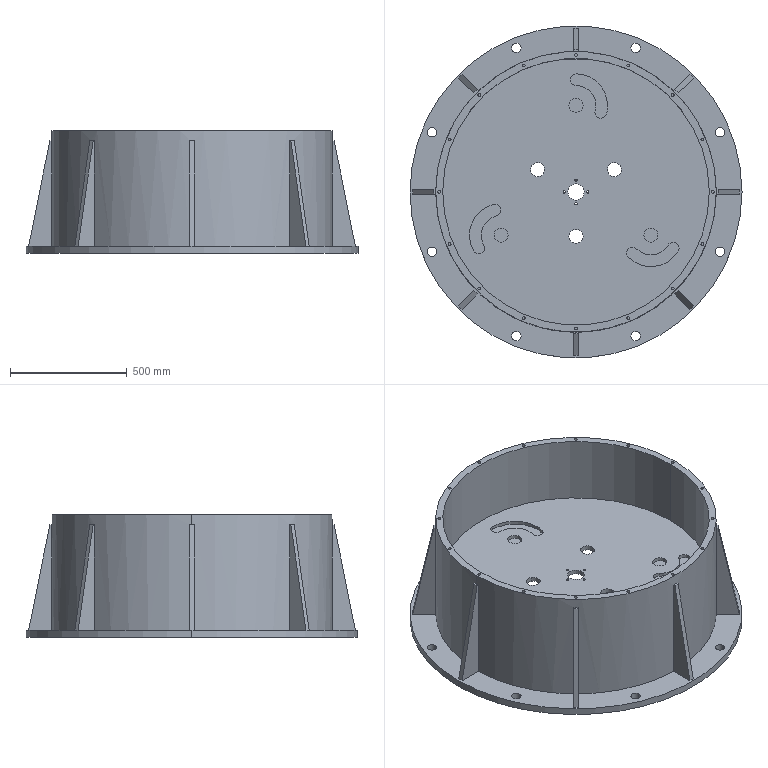Part | SolidWorks | features ICE 7, CirPattern 2, Cut 1, Extrusion 1 | 1 solid | 154 faces | box 1420 x 1420 x 525 mm | volume 94468216 mm3 | cylinder 95 | plane 59 | commonest cylinder face diameters 12 x32 40 x16 60 x12 50 x9 10 x8 170 x4